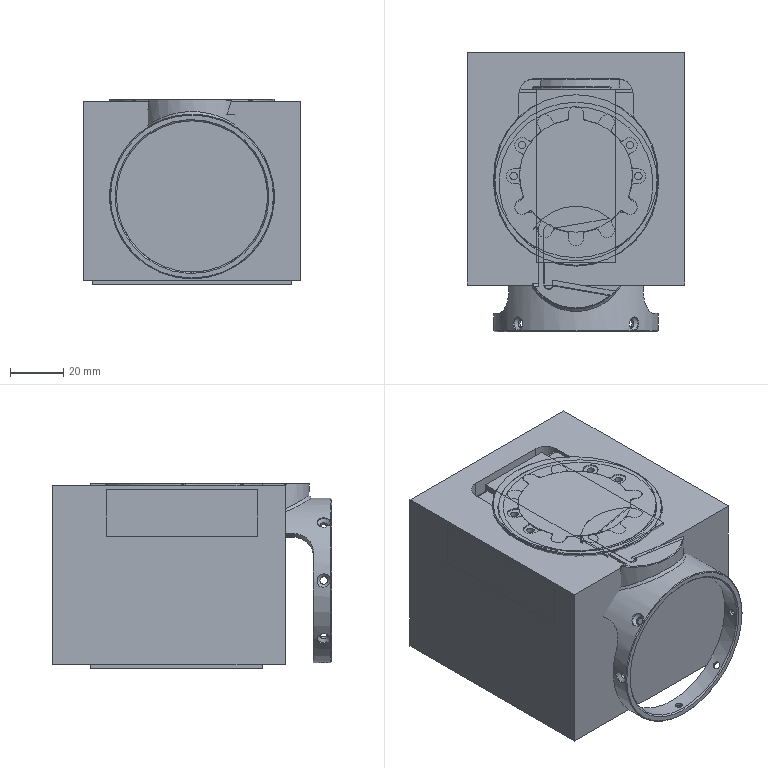NC program | NX | posted with a generic post | part box 82 x 105.2 x 70 mm
Lines 901 to 1807 of 123648:
(外形动态铣_COPY , TOOL : 粗刀D10)
N1782 T15 M6
N1784 G53
N1786 G18 G0 G90 X2.248 Z-25.338 S8500 M3
N1788 G43 Y78.5 H15
N1790 G94 G1 Y34.864 F3500.
N1792 X2.295 Y34.857 Z-25.155
N1794 X2.305 Y34.856 Z-25.13
N1796 X2.322 Y34.855 Z-25.11
N1798 X2.344 Y34.854 Z-25.095
N1800 X2.369 Y34.853 Z-25.088
N1802 X2.396 Y34.852
N1804 X2.421 Y34.851 Z-25.095
N1806 X2.443 Z-25.11
N1808 G3 X2.443 Y34.033 Z-25.11 I-2.424 K-2.83
N1810 X2.443 Y33.215 Z-25.11 I-2.424 K-2.83
N1812 X2.443 Y32.398 Z-25.11 I-2.424 K-2.83
N1814 X2.443 Y31.58 Z-25.11 I-2.424 K-2.83
N1816 X2.443 Y30.762 Z-25.11 I-2.424 K-2.83
N1818 X2.443 Y29.945 Z-25.11 I-2.424 K-2.83
N1820 X2.443 Y29.127 Z-25.11 I-2.424 K-2.83
N1822 X2.443 Y28.309 Z-25.11 I-2.424 K-2.83
N1824 X2.443 Y27.492 Z-25.11 I-2.424 K-2.83
N1826 X2.443 Y26.674 Z-25.11 I-2.424 K-2.83
N1828 X2.443 Y25.856 Z-25.11 I-2.424 K-2.83
N1830 X2.443 Y25.039 Z-25.11 I-2.424 K-2.83
N1832 X2.443 Y24.221 Z-25.11 I-2.424 K-2.83
N1834 X2.443 Y23.403 Z-25.11 I-2.424 K-2.83
N1836 X2.443 Y22.586 Z-25.11 I-2.424 K-2.83
N1838 X2.443 Y21.768 Z-25.11 I-2.424 K-2.83
N1840 X2.443 Y20.95 Z-25.11 I-2.424 K-2.83
N1842 X2.443 Y20.133 Z-25.11 I-2.424 K-2.83
N1844 X2.443 Y19.315 Z-25.11 I-2.424 K-2.83
N1846 X2.443 Y18.497 Z-25.11 I-2.424 K-2.83
N1848 X2.443 Y17.68 Z-25.11 I-2.424 K-2.83
N1850 X2.443 Y16.862 Z-25.11 I-2.424 K-2.83
N1852 X2.443 Y16.044 Z-25.11 I-2.424 K-2.83
N1854 X3.745 Y15.93 Z-28.001 R3.727
N1856 X3.745 Z-27.96 R-3.748
N1858 G1 X3.778 Z-28.081
N1860 X3.79 Z-28.205
N1862 X3.795 Z-28.231
N1864 G3 X1.945 Z-31.269 R3.792
N1866 X-2.771 Z-30.609 R3.819
N1868 X-3.768 Z-28.538 R3.906
N1870 X-0.169 Z-24.196 R3.816
N1872 X2.469 Z-25.105 R3.845
N1874 X3.293 Z-26.089 R4.24
N1876 X3.793 Z-28.262 R3.828
N1878 X3.166 Z-28.712 R0.505
N1880 G1 X1.594 Z-28.316
N1882 Y16.93
N1884 G0 Y78.5
N1886 X29.527 Z-4.88
N1888 G1 Y19.899
N1890 Y18.899
N1892 G3 X29.287 Z-5.852 R-0.505
N1894 G1 X27.657 Z-5.215
N1896 G3 X27.345 Z-4.842 R0.505
N1898 X27.07 Z-3.887 R14.618
N1900 G1 X27.042 Z-3.804
N1902 G3 X26.84 Z-3.011 R8.746
N1904 X26.876 Z-2.627 R0.799
N1906 G2 X27.225 Z-1.531 R5.794
N1908 G1 X27.344 Z-1.173
N1910 X27.352 Z-1.115
N1912 X27.344 Z-1.173
N1914 G2 X27.175 Z-1.747 R3.561
N1916 G3 X26.876 Z-2.627 R5.632
N1918 G2 X26.768 Z-3.082 R0.871
N1920 X26.918 Z-3.475 R1.353
N1922 G1 X27.042 Z-3.804
N1924 G2 X27.892 Z-3.962 R0.505
N1926 G1 X28.397 Z-3.393
N1928 G3 X29.279 Z-3.726 R0.505
N1930 G1 Y19.899
N1932 G0 Y78.5
N1934 X29.067 Z-5.02
N1936 G1 Y20.394
N1938 Y19.394
N1940 G3 X28.826 Z-5.992 R-0.505
N1942 G1 X27.198 Z-5.358
N1944 G3 X26.886 Z-4.985 R0.505
N1946 X26.719 Z-4.45 R15.136
N1948 G2 X26.532 Z-3.77 R4.464
N1950 G3 X26.34 Z-2.921 R8.059
N1952 X26.373 Z-2.645 R0.907
N1954 G2 X26.736 Z-1.479 R5.658
N1956 G1 X26.885 Z-1.03
N1958 X26.892 Z-0.971
N1960 X26.885 Z-1.03
N1962 G2 X26.68 Z-1.745 R4.244
N1964 G3 X26.373 Z-2.645 R5.523
N1966 G2 X26.275 Z-3.083 R0.804
N1968 X26.423 Z-3.475 R1.395
N1970 G1 X26.554 Z-3.827
N1972 G2 X27.379 Z-4.013 R0.505
N1974 G1 X27.953 Z-3.456
N1976 G3 X28.81 Z-3.815 R0.505
N1978 G1 Y20.394
N1980 G0 Y78.5
N1982 X28.656 Z-5.851
N1984 G1 Y20.888
N1986 Y19.888
N1988 G2 X28.744 Z-4.797 R-0.529
N1990 G1 X26.939 Z-4.685
N1992 G3 X26.48 Z-4.351 R0.529
N1994 G1 X26.468 Z-4.321
N1996 X26.167 Z-3.774
N1998 G3 X25.939 Z-2.813 R3.831
N2000 X26.012 Z-2.509 R0.818
N2002 G1 X26.47 Z-1.632
N2004 X26.48 Z-1.606
N2006 X26.47 Z-1.632
N2008 X26.012 Z-2.509
N2010 G2 X25.854 Z-3.04 R1.2
N2012 X25.983 Z-3.439 R0.961
N2014 G1 X26.224 Z-3.877
N2016 G2 X27.094 Z-3.904 R0.505
N2018 G1 X27.533 Z-3.208
N2020 G3 X28.465 Z-3.475 R0.505
N2022 G1 Y20.888
N2024 G0 Y78.5
N2026 X28.308 Z-4.565
N2028 G1 Y21.383
N2030 Y20.383
N2032 G2 X27.409 Z-4.22 R0.505
N2034 G1 X27.001 Z-4.732
N2036 G3 X26.132 Z-4.59 R0.505
N2038 X25.662 Z-3.658 R36.06
N2040 G1 X25.607 Z-3.452
N2042 G3 X25.532 Z-2.922 R2.623
N2044 G1 X25.548 Z-2.786
N2046 G2 X25.764 Z-1.296 R6.024
N2048 X25.744 Z0.158 R22.27
N2050 X23.618 Z3.888 R5.207
N2052 X22.281 Z4.703 R10.28
N2054 X21.487 Z4.989 R4.809
N2056 G3 X22.984 Z4.312 R5.372
N2058 X24.143 Z3.456 R8.234
N2060 X25.763 Z-0.441 R5.229
N2062 X25.742 Z-1.747 R17.885
N2064 X25.548 Z-2.786 R6.162
N2066 G2 X25.536 Z-3.207 R0.736
N2068 G1 X25.607 Z-3.452
N2070 G2 X26.03 Z-3.813 R0.505
N2072 G1 X27.616 Z-4.01
N2074 G2 X27.767 Z-3.012 R0.505
N2076 G1 Y21.383
N2078 G0 Y78.5
N2080 X30.042 Z-58.825
N2082 G1 Y19.404
N2084 Y18.404
N2086 G3 X30.341 Z-59.935 R0.586
N2088 G1 X28.506 Z-60.856
N2090 G3 X27.814 Z-60.731 R0.586
N2092 X27.604 Z-60.279 R2.401
N2094 X27.657 Z-59.848 R0.81
N2096 G1 X27.8 Z-59.618
N2098 X27.81 Z-59.595
N2100 X27.8 Z-59.618
N2102 X27.591 Z-59.954
N2104 G2 X27.48 Z-60.428 R1.361
N2106 X27.604 Z-60.774 R0.524
N2108 X27.868 Z-60.989 R0.65
N2110 G1 X27.849 Z-60.986
N2112 X27.835 Z-60.983
N2114 X27.814 Z-60.976
N2116 G3 X27.494 Z-60.109 R0.566
N2118 G1 X27.626 Z-59.897
N2120 G3 X27.85 Z-59.699 R0.529
N2122 G1 X29.985 Z-58.695
N2124 Y19.404
N2126 G0 Y78.5
N2128 X29.567 Z-58.825
N2130 G1 Y19.899
N2132 Y18.899
N2134 G3 X29.437 Z-59.234 R0.586
N2136 G1 X28.234 Z-60.714
N2138 G3 X27.349 Z-60.742 R0.586
N2140 X27.146 Z-60.32 R2.797
N2142 X27.174 Z-59.848 R0.752
N2144 G1 X27.335 Z-59.584
N2146 X27.345 Z-59.558
N2148 X27.335 Z-59.584
N2150 X27.11 Z-59.955
N2152 G2 X27.017 Z-60.539 R1.208
N2154 X27.457 Z-60.998 R0.662
N2156 G1 X27.349 Z-60.98
N2158 G3 X27.013 Z-60.116 R0.567
N2160 G1 X27.142 Z-59.902
N2162 G3 X27.663 Z-59.65 R0.531
N2164 G1 X29.497 Z-59.882
N2166 G2 X29.567 Z-58.825 R-0.531
N2168 G1 Y19.899
N2170 G0 Y78.5
N2172 X29.202 Z-58.823
N2174 G1 Y20.394
N2176 Y19.394
N2178 G3 X29.058 Z-59.256 R0.605
N2180 G1 X27.786 Z-60.746
N2182 G3 X26.892 Z-60.774 R0.605
N2184 X26.577 Z-60.022 R2.95
N2186 X26.584 Z-59.73 R1.193
N2188 G2 X26.73 Z-59.172 R8.097
N2190 G1 X26.884 Z-58.682
N2192 X26.892 Z-58.621
N2194 X26.884 Z-58.682
N2196 G2 X26.613 Z-59.643 R8.144
N2198 G1 X26.543 Z-59.848
N2200 G2 X26.495 Z-60.558 R1.711
N2202 X26.945 Z-61. R0.664
N2204 G1 X26.892 Z-60.997
N2206 X26.744 Z-60.967
N2208 G3 X26.391 Z-60.481 R0.64
N2210 G1 X26.383 Z-60.293
N2212 X26.555 Z-59.815
N2214 X26.383 Z-60.293
N2216 G2 X26.744 Z-60.967 R0.561
N2218 X27.157 Z-60.941 R0.636
N2220 G1 X29.309 Z-60.045
N2222 G2 X29.092 Z-58.823 R0.636
N2224 G1 Y20.394
N2226 G0 Y78.5
N2228 X28.792
N2230 G1 Y20.888
N2232 Y19.888
N2234 G3 X28.627 Z-59.287 R0.623
N2236 G1 X27.243 Z-60.783
N2238 G3 X26.462 Z-60.893 R0.623
N2240 X26.314 Z-60.693 R0.578
N2242 X26.072 Z-59.911 R4.395
N2244 X26.093 Z-59.648 R0.932
N2246 G2 X26.277 Z-58.716 R5.664
N2248 G3 X26.478 Z-58.083 R7.143
N2250 G1 X26.485 Z-58.025
N2252 X26.478 Z-58.083
N2254 G2 X26.277 Z-58.716 R7.143
N2256 G3 X26.093 Z-59.648 R5.664
N2258 G1 X26.013 Z-59.885
N2260 G2 X26.012 Z-60.517 R1.917
N2262 X26.295 Z-60.91 R0.55
N2264 G1 X26.503 Z-61.
N2266 X26.431
N2268 X26.374 Z-60.997
N2270 X26.352 Z-60.995
N2272 X26.235 Z-60.953
N2274 G3 X25.972 Z-60.681 R1.494
N2276 X25.889 Z-60.321 R0.58
N2278 G1 X25.911 Z-60.157
N2280 X25.947 Z-60.075
N2282 X25.957 Z-60.051
N2284 X26.037 Z-59.814
N2286 X25.957 Z-60.051
N2288 X25.947 Z-60.075
N2290 X25.911 Z-60.157
N2292 G2 X26.352 Z-60.995 R0.573
N2294 X26.641 Z-60.949 R0.631
N2296 G1 X28.846 Z-60.036
N2298 G2 X28.64 Z-58.823 R0.631
N2300 G1 Y20.888
N2302 G0 Y78.5
N2304 X28.363 Z-58.825
N2306 G1 Y21.383
N2308 Y20.383
N2310 G3 X28.632 Z-60.019 R0.622
N2312 G1 X26.416 Z-60.955
N2314 G3 X26.004 Z-60.917 R0.46
N2316 G1 X25.908 Z-60.836
N2318 G3 X25.742 Z-60.423 R1.485
N2320 X25.584 Z-59.686 R7.721
N2322 G1 X25.585 Z-59.522
N2324 G2 X25.763 Z-58.404 R5.443
N2326 G1 X25.795 Z-58.269
N2328 X26.13 Z-57.261
N2330 X26.138 Z-57.203
N2332 X26.13 Z-57.261
N2334 X25.776 Z-58.338
N2336 G2 X25.731 Z-58.775 R4.176
N2338 G3 X25.585 Z-59.522 R5.461
N2340 G1 X25.563 Z-59.618
N2342 X25.555 Z-59.644
N2344 X25.514 Z-59.763
N2346 G2 X25.568 Z-60.625 R1.514
N2348 X25.923 Z-60.955 R0.574
N2350 G1 X26.074 Z-61.
N2352 X26.199
N2354 X25.949
N2356 X25.826 Z-60.977
N2358 X25.627 Z-60.839
N2360 G3 X25.417 Z-60.541 R1.294
N2362 X25.384 Z-60.129 R0.836
N2364 G1 X25.408 Z-60.07
N2366 X25.413 Z-60.057
N2368 X25.535 Z-59.702
N2370 X25.413 Z-60.057
N2372 X25.408 Z-60.07
N2374 X25.384 Z-60.129
N2376 G2 X25.478 Z-60.836 R0.609
N2378 X25.891 Z-61. R0.589
N2380 G1 X26.016
N2382 G2 X26.459 Z-60.795 R0.582
N2384 G1 X27.812 Z-59.201
N2386 G2 X27.951 Z-58.825 R0.582
N2388 G1 Y21.383
N2390 G0 Y78.5
N2392 X28.115 Z-58.823
N2394 G1 Y21.878
N2396 Y20.878
N2398 G3 X28.369 Z-60.051 R0.636
N2400 G1 X26.012 Z-60.958
N2402 G3 X25.446 Z-60.892 R0.605
N2404 G1 X25.294 Z-60.683
N2406 G3 X25.087 Z-59.212 R7.832
N2408 G2 X25.187 Z-57.904 R5.906
N2410 G1 X25.193 Z-3.464
N2412 G2 X25.178 Z0.004 R213.685
N2414 X23.973 Z3.026 R5.21
N2416 X22.723 Z4.106 R5.746
N2418 X21.598 Z4.749 R7.672
N2420 X20.859 Z5.003 R5.58
N2422 G3 X20.981 Z5.987 R0.5
N2424 G1 X21.893
N2426 X23.493 Y21.378
N2428 X24.17 Z5.984 F15000.
N2430 X24.336 Z5.934
N2432 X24.907 Z5.653
N2434 X25.469 Z5.353
N2436 G3 X26.515 Z4.119 R2.718
N2438 G1 X27.493 Z1.804
N2440 G3 X28.263 Z-2.383 R11.082
N2442 G1 X27.628 Z-56.727
N2444 G3 X27.46 Z-57.039 R0.511
N2446 G1 X27.191 Z-57.271
N2448 X25.98 Y20.878 Z-58.317 F3500.
N2450 X25.246 Z-58.952
N2452 G2 X25.087 Z-59.212 R0.5
N2454 G1 X24.988 Z-59.621
N2456 X24.982 Z-59.642
N2458 G2 X24.96 Z-60.397 R1.665
N2460 X25.098 Z-60.736 R1.339
N2462 X25.516 Z-60.986 R0.616
N2464 G1 X25.566 Z-61.
N2466 X25.816
N2468 X25.441
N2470 X25.318 Z-60.981
N2472 X25.108 Z-60.847
N2474 G3 X24.878 Z-60.548 R1.841
N2476 X24.858 Z-60.015 R0.726
N2478 G1 X24.878 Z-59.958
N2480 X24.882 Z-59.948
N2482 X24.982 Z-59.642
N2484 X24.882 Z-59.948
N2486 X24.878 Z-59.958
N2488 X24.842 Z-60.055
N2490 X24.836 Z-60.071
N2492 X24.789 Z-60.178
N2494 X24.76 Z-60.299
N2496 G2 X24.832 Z-60.659 R1.287
N2498 X25.092 Z-60.921 R0.564
N2500 G1 X25.279 Z-60.998
N2502 X25.318 Z-61.
N2504 X25.443
N2506 X25.318
N2508 X25.279 Z-60.998
N2510 G3 X24.789 Z-60.178 R0.569
N2512 X25.048 Z-59.908 R0.588
N2514 G1 X27.339 Z-58.714
N2516 Y21.878
N2518 G0 Y78.5
N2520 X27.499 Z-58.823
N2522 G1 Y22.373
N2524 Y21.373
N2526 G3 X27.756 Z-60.034 R0.628
N2528 G1 X25.451 Z-60.955
N2530 G3 X24.878 Z-60.902 R0.633
N2532 G1 X24.724 Z-60.702
N2534 G3 X24.526 Z-59.641 R7.264
N2536 X24.494 Z-59.174 R1.883
N2538 G2 X24.588 Z-57.904 R5.87
N2540 G1 X24.595 Z-32.861
N2542 G3 X24.66 Z-31.981 R7.101
N2544 G2 X24.679 Z-24.203 R39.152
N2546 G1 X24.595 Z-23.298
N2548 X24.588 Z-0.441
N2550 G2 X22.29 Z3.991 R5.19
N2552 X21.413 Z4.536 R17.777
N2554 X20.188 Z5.015 R5.079
N2556 G3 X20.153 Z5.965 R0.5
N2558 G1 X20.294 Z6.017
N2560 X21.796 Y21.873 Z6.569
N2562 X22.84 Z6.948 F15000.
N2564 G3 X23.306 Z6.815 R0.503
N2566 G1 X26.557 Z3.557
N2568 G3 X27.306 Z1.608 R2.915
N2570 G1 X27.303 Z-14.519
N2572 X27.28 Z-23.185
N2574 X27.234 Z-31.852
N2576 X27.035 Z-56.69
N2578 G3 X26.863 Z-57.006 R0.51
N2580 G1 X26.592 Z-57.236
N2582 X25.371 Y21.373 Z-58.27 F3500.
N2584 X24.665 Z-58.87
N2586 G2 X24.494 Z-59.174 R0.5
N2588 G3 X24.382 Z-59.641 R4.804
N2590 G2 X24.48 Z-60.692 R1.54
N2592 X24.875 Z-60.976 R0.596
N2594 G1 X24.964 Z-61.
N2596 X25.339
N2598 X24.839
N2600 X24.716 Z-60.979
N2602 X24.503 Z-60.832
N2604 G3 X24.285 Z-60.553 R1.705
N2606 X24.252 Z-60.025 R0.725
N2608 G1 X24.382 Z-59.641
N2610 X24.244 Z-60.051
N2612 X24.234 Z-60.075
N2614 X24.189 Z-60.177
N2616 X24.16 Z-60.299
N2618 G2 X24.231 Z-60.653 R1.378
N2620 X24.487 Z-60.918 R0.562
N2622 G1 X24.677 Z-60.998
N2624 X24.718 Z-61.
N2626 X24.843
N2628 X24.718
N2630 X24.677 Z-60.998
N2632 G3 X24.189 Z-60.177 R0.569
N2634 X24.447 Z-59.909 R0.589
N2636 G1 X26.741 Z-58.703
N2638 Y22.373
N2640 G0 Y78.5
N2642 X26.889 Z-58.823
N2644 G1 Y22.868
N2646 Y21.868
N2648 G3 X27.147 Z-60.031 R0.627
N2650 G1 X24.852 Z-60.955
N2652 G3 X24.278 Z-60.902 R0.633
N2654 G1 X24.124 Z-60.702
N2656 G3 X23.926 Z-59.641 R7.224
N2658 G1 X23.871 Z-59.137
N2660 G2 X23.962 Z-57.903 R5.538
N2662 G1 X23.964 Z-35.457
N2664 G3 X24.063 Z-34.573 R3.822
N2666 G2 X24.466 Z-31.548 R39.464
N2668 X24.675 Z-28.95 R47.216
N2670 X24.603 Z-25.933 R25.491
N2672 X24.23 Z-22.475 R64.034
N2674 G1 X24.014 Z-21.141
N2676 X23.965 Z-20.693
N2678 X23.962 Z-0.441
N2680 G2 X22.283 Z3.506 R5.217
N2682 X21.418 Z4.149 R6.
N2684 X20.327 Z4.749 R9.712
N2686 X19.594 Z5.001 R6.662
N2688 G3 X19.543 Z5.957 R0.5
N2690 G1 X19.681 Z6.007
N2692 X21.185 Y22.368 Z6.553
N2694 X22.248 Z6.935 F15000.
N2696 G3 X22.712 Z6.801 R0.503
N2698 G1 X25.946 Z3.562
N2700 G3 X26.726 Z1.576 R3.01
N2702 G1 X26.951 Z-17.779
N2704 G3 X26.753 Z-42.894 R755.168
N2706 G1 X26.411 Z-56.651
N2708 G3 X26.241 Z-56.96 R0.511
N2710 G1 X25.965 Z-57.195
N2712 X24.748 Y21.868 Z-58.233 F3500.
N2714 X24.04 Z-58.836
N2716 G2 X23.871 Z-59.137 R0.5
N2718 G1 X23.754 Z-59.643
N2720 G2 X23.856 Z-60.675 R1.627
N2722 X24.365 Z-60.993 R0.62
N2724 G1 X24.39 Z-61.
N2726 X24.64
N2728 X24.265
N2730 X24.14 Z-60.988
N2732 X23.93 Z-60.87
N2734 G3 X23.634 Z-60.484 R1.37
N2736 X23.61 Z-60.07 R0.817
N2738 G1 X23.615 Z-60.056
N2740 X23.754 Z-59.643
N2742 X23.615 Z-60.056
N2744 X23.61 Z-60.07
N2746 X23.587 Z-60.129
N2748 X23.581 Z-60.142
N2750 X23.568 Z-60.17
N2752 X23.539 Z-60.292
N2754 G2 X23.607 Z-60.642 R1.435
N2756 X23.858 Z-60.913 R0.56
N2758 G1 X24.053 Z-60.998
N2760 X24.095 Z-61.
N2762 X24.345
N2764 X24.095
N2766 X24.053 Z-60.998
N2768 G3 X23.568 Z-60.17 R0.569
N2770 X23.823 Z-59.91 R0.587
N2772 G1 X26.114 Z-58.714
N2774 Y22.868
N2776 G0 Y78.5
N2778 X26.247 Z-58.823
N2780 G1 Y23.362
N2782 Y22.362
N2784 G3 X26.215 Z-59.911 R0.625
N2786 G1 X24.281 Z-60.928
N2788 G3 X23.651 Z-60.895 R0.615
N2790 G1 X23.499 Z-60.698
N2792 G3 X23.302 Z-59.639 R7.309
N2794 G1 X23.226 Z-59.004
N2796 G2 X23.294 Z-57.904 R5.912
N2798 G1 X23.297 Z-37.231
N2800 G3 X23.467 Z-36.302 R5.471
N2802 G2 X23.821 Z-34.551 R40.838
N2804 X24.448 Z-31.444 R31.314
N2806 X23.843 Z-21.579 R24.764
N2808 X23.425 Z-19.517 R37.831
N2810 G3 X23.3 Z-18.726 R13.405
N2812 G1 X23.294 Z-0.441
N2814 G2 X20.985 Z3.999 R5.193
N2816 X19.641 Z4.749 R11.461
N2818 X18.959 Z4.994 R6.353
N2820 G3 X19.056 Z5.985 R0.5
N2822 G1 X19.976 Z5.983
N2824 X21.576 Y22.862 Z5.98
N2826 X22.271 Z5.975 F15000.
N2828 X22.436 Z5.926
N2830 X23.007 Z5.645
N2832 X23.568 Z5.344
N2834 G3 X24.605 Z4.107 R2.669
N2836 G1 X25.555 Z1.78
N2838 G3 X26.252 Z-2.356 R10.761
N2840 G1 X25.84 Z-16.242
N2842 G3 X25.662 Z-16.554 R0.51
N2844 G1 X25.302 Z-16.846
N2846 X24.061 Y22.362 Z-17.855 F3500.
N2848 X23.485 Z-18.324
N2850 G2 X23.3 Z-18.726 R0.5
N2852 X23.328 Z-19.099 R1.646
N2854 G1 X23.437 Z-19.572
N2856 G2 X23.735 Z-19.924 R0.5
N2858 G1 X24.238 Z-20.131
N2860 X25.718 Y22.862 Z-20.739
N2862 X26.302 Z-20.982 F15000.
N2864 G3 X26.555 Z-21.372 R0.503
N2866 G1 X26.748 Z-23.407
N2868 X26.919 Z-25.443
N2870 G3 X26.971 Z-30.339 R43.519
N2872 G1 X25.765 Z-56.517
N2874 G3 X25.597 Z-56.816 R0.513
N2876 G1 X25.295 Z-57.074
N2878 X24.08 Y22.362 Z-58.115 F3500.
N2880 X23.395 Z-58.701
N2882 G2 X23.226 Z-59.004 R0.5
N2884 G3 X23.094 Z-59.621 R3.815
N2886 G2 X23.212 Z-60.657 R1.674
N2888 X23.71 Z-60.991 R0.611
N2890 G1 X23.743 Z-61.
N2892 X24.118
N2894 X23.618
N2896 X23.494 Z-60.986
N2898 X23.279 Z-60.856
N2900 G3 X22.975 Z-60.452 R1.582
N2902 X22.95 Z-60.04 R0.832
N2904 G1 X23.087 Z-59.641
N2906 X23.094 Z-59.621
N2908 X22.893 Z-60.19
N2910 G2 X22.968 Z-60.671 R1.175
N2912 X23.234 Z-60.927 R0.565
N2914 G1 X23.423 Z-61.
N2916 X23.673
N2918 X23.423
N2920 G3 X22.891 Z-60.18 R0.572
N2922 G1 X22.938 Z-60.073
N2924 G3 X23.21 Z-59.788 R0.574
N2926 G1 X25.448 Z-58.686
N2928 Y23.362
N2930 G0 Y78.5
N2932 X25.562 Z-58.823
N2934 G1 Y23.857
N2936 Y22.857
N2938 G3 X25.538 Z-59.911 R0.623
N2940 G1 X23.611 Z-60.928
N2942 G3 X22.981 Z-60.896 R0.616
N2944 G1 X22.827 Z-60.697
N2946 G3 X22.631 Z-59.642 R7.117
N2948 X22.543 Z-58.831 R14.807
N2950 G2 X22.585 Z-57.903 R6.27
N2952 G1 X22.592 Z-38.939
N2954 G3 X22.764 Z-38.03 R3.172
N2956 G1 X23.117 Z-36.699
N2958 G2 X24.118 Z-33.278 R28.314
N2960 X23.143 Z-19.387 R24.753
N2962 G1 X22.835 Z-18.224
N2964 G3 X22.592 Z-16.75 R13.55
N2966 G1 X22.585 Z-0.441
N2968 G2 X21.367 Z3.025 R5.21
N2970 X19.751 Z4.313 R5.59
N2972 X18.826 Z4.786 R7.766
N2974 X18.197 Z4.998 R5.071
N2976 G3 X18.137 Z5.956 R0.5
N2978 G1 X18.27 Z6.004
N2980 X19.775 Y23.357 Z6.548
N2982 X20.852 Z6.933 F15000.
N2984 G3 X21.315 Z6.798 R0.503
N2986 G1 X24.577 Z3.531
N2988 G3 X25.303 Z1.608 R2.833
N2990 G1 X25.133 Z-14.266
N2992 G3 X24.953 Z-14.586 R0.509
N2994 G1 X24.6 Z-14.874
N2996 X23.36 Y22.857 Z-15.886 F3500.
N2998 X22.776 Z-16.362
N3000 G2 X22.592 Z-16.75 R0.5
N3002 X22.614 Z-17.383 R3.663
N3004 X22.848 Z-18.276 R10.518
N3006 X23.763 Z-18.413 R0.505
N3008 G1 X24.123 Z-17.842
N3010 G3 X25.055 Z-18.106 R0.505
N3012 G1 Y23.857
N3014 G0 Y78.5
N3016 X24.831 Z-58.823
N3018 G1 Y23.857
N3020 Y22.857
N3022 G3 X24.757 Z-59.133 R0.528
N3024 G1 X23.789 Z-60.744
N3026 G3 X23.336 Z-61. R0.528
N3028 G1 X23.211
N3030 G3 X22.972 Z-60.935 R0.541
N3032 X22.545 Z-60.39 R1.862
N3034 G1 X22.435 Z-60.175
N3036 G3 X22.369 Z-59.669 R0.744
N3038 G2 X22.546 Z-58.817 R4.874
N3040 G3 X22.369 Z-59.669 R4.874
N3042 G1 X22.331 Z-59.788
N3044 X22.303 Z-59.91
N3046 G2 X22.494 Z-60.708 R1.586
N3048 X22.898 Z-60.98 R0.603
N3050 G1 X22.97 Z-61.
N3052 X23.22
N3054 X22.845
N3056 X22.722 Z-60.979
N3058 X22.519 Z-60.848
N3060 G3 X22.278 Z-60.555 R1.908
N3062 X22.232 Z-60.07 R0.723
N3064 G1 X22.366 Z-59.678
N3066 X22.232 Z-60.07
N3068 X22.185 Z-60.178
N3070 X22.156 Z-60.299
N3072 G2 X22.225 Z-60.648 R1.268
N3074 X22.479 Z-60.916 R0.561
N3076 G1 X22.671 Z-60.998
N3078 X22.714 Z-61.
N3080 X22.964
N3082 X22.714
N3084 X22.671 Z-60.998
N3086 G3 X22.185 Z-60.178 R0.569
N3088 X22.451 Z-59.906 R0.583
N3090 G1 X24.733 Z-58.765
N3092 Y23.857
N3094 G0 Y78.5
N3096 X24.836 Z-58.823
N3098 G1 Y24.352
N3100 Y23.352
N3102 G3 X24.82 Z-59.909 R0.62
N3104 G1 X22.905 Z-60.928
N3106 G3 X22.274 Z-60.902 R0.628
N3108 G1 X22.119 Z-60.702
N3110 G3 X21.922 Z-59.642 R7.204
N3112 X21.813 Z-58.624 R21.224
N3114 G2 X21.834 Z-57.903 R5.787
N3116 G1 X21.843 Z-40.22
N3118 G3 X21.944 Z-39.757 R1.197
N3120 G1 X22.373 Z-38.445
N3122 G3 X22.655 Z-37.844 R6.373
N3124 G1 X22.913 Z-37.458
N3126 G2 X23.117 Z-36.699 R10.669
N3128 X24.118 Z-33.278 R28.314
N3130 X23.143 Z-19.387 R24.753
N3132 G1 X22.919 Z-18.538
N3134 G2 X22.598 Z-18.041 R7.171
N3136 G3 X22.211 Z-17.048 R6.241
N3138 X21.842 Z-14.831 R13.553
N3140 G1 X21.834 Z-0.441
N3142 G2 X19.256 Z4.162 R5.189
N3144 X17.958 Z4.822 R11.328
N3146 G1 X17.433 Z4.996
N3148 G3 X17.37 Z5.955 R0.5
N3150 G1 X17.499 Z6.001
N3152 X19.004 Y23.852 Z6.544
N3154 X20.088 Z6.93 F15000.
N3156 G3 X20.55 Z6.796 R0.503
N3158 G1 X23.813 Z3.528
N3160 G3 X24.538 Z1.606 R2.831
N3162 G1 X24.383 Z-12.348
N3164 G3 X24.204 Z-12.667 R0.509
N3166 G1 X23.847 Z-12.958
N3168 X22.607 Y23.352 Z-13.969 F3500.
N3170 X22.026 Z-14.443
N3172 G2 X21.842 Z-14.831 R0.5
N3174 X21.859 Z-15.937 R16.442
N3176 X22.007 Z-16.426 R3.027
N3178 G1 X22.227 Z-17.096
N3180 G2 X23.148 Z-17.19 R0.505
N3182 G1 X23.492 Z-16.58
N3184 G3 X24.436 Z-16.823 R0.505
N3186 G1 Y24.352
N3188 G0 Y78.5
N3190 X24.098 Z-58.823
N3192 G1 Y24.352
N3194 Y23.352
N3196 G3 X24.027 Z-59.126 R0.525
N3198 G1 X23.083 Z-60.74
N3200 G3 X22.629 Z-61. R0.525
N3202 G1 X22.504
N3204 G3 X22.264 Z-60.936 R0.539
N3206 X21.836 Z-60.389 R1.865
N3208 X21.63 Z-59.94 R2.331
N3210 X21.626 Z-59.645 R0.871
N3212 G2 X21.821 Z-58.506 R4.888
N3214 G3 X21.626 Z-59.645 R4.888
N3216 G1 X21.586 Z-59.764
N3218 G2 X21.577 Z-60.136 R1.075
N3220 X21.784 Z-60.723 R1.711
N3222 X22.196 Z-60.983 R0.609
N3224 G1 X22.255 Z-61.
N3226 X22.505
N3228 X22.13
N3230 X22.007 Z-60.98
N3232 G3 X21.557 Z-60.573 R1.257
N3234 X21.48 Z-60.076 R0.732
N3236 G1 X21.482 Z-60.071
N3238 X21.488 Z-60.055
N3240 X21.608 Z-59.7
N3242 X21.488 Z-60.055
N3244 X21.482 Z-60.071
N3246 X21.434 Z-60.188
N3248 X21.41 Z-60.31
N3250 G2 X21.496 Z-60.659 R1.269
N3252 X21.755 Z-60.921 R0.562
N3254 G1 X21.946 Z-60.999
N3256 X21.968 Z-61.
N3258 X22.218
N3260 X21.968
N3262 X21.946 Z-60.999
N3264 G3 X21.434 Z-60.188 R0.57
N3266 X21.711 Z-59.9 R0.581
N3268 G1 X23.981 Z-58.793
N3270 Y24.352
N3272 G0 Y78.5
N3274 X24.065 Z-58.823
N3276 G1 Y24.847
N3278 Y23.847
N3280 G3 X23.877 Z-59.308 R0.616
N3282 G1 X22.295 Z-60.828
N3284 G3 X21.528 Z-60.896 R0.613
N3286 G1 X21.374 Z-60.697
N3288 G3 X21.176 Z-59.637 R7.319
N3290 X21.034 Z-58.254 R24.101
N3292 G1 X21.047 Z-41.434
N3294 X21.094 Z-41.246
N3296 X21.484 Z-40.232
N3298 G3 X21.92 Z-39.387 R8.71
N3300 G1 X22.172 Z-39.047
N3302 X22.197 Z-38.995
N3304 G3 X23.131 Z-39.075 R0.5
N3306 G1 X23.519 Y24.347 Z-40.627
N3308 X23.767 Z-41.63 F15000.
N3310 X23.772 Z-41.723
N3312 X23.256 Z-56.089
N3314 G3 X23.039 Z-56.428 R0.518
N3316 G1 X21.784 Y23.847 Z-57.421 F3500.
N3318 X21.224 Z-57.865
N3320 G2 X21.034 Z-58.254 R0.5
N3322 G3 X20.905 Z-59.331 R4.75
N3324 G2 X20.897 Z-60.236 R2.225
N3326 X21.137 Z-60.778 R1.471
N3328 X21.576 Z-60.993 R0.643
N3330 G1 X21.601 Z-61.
N3332 X21.976
N3334 X21.476
N3336 X21.352 Z-60.988
N3338 X21.128 Z-60.863
N3340 G3 X20.758 Z-60.378 R1.549
N3342 X20.721 Z-59.957 R0.825
N3344 G1 X20.828 Z-59.643
N3346 X20.835 Z-59.619
N3348 X20.924 Z-59.254
N3350 X20.835 Z-59.619
N3352 X20.828 Z-59.643
N3354 X20.688 Z-60.054
N3356 X20.681 Z-60.072
N3358 X20.656 Z-60.195
N3360 G2 X20.84 Z-60.763 R1.094
N3362 X21.281 Z-61. R0.731
N3364 G1 X21.531
N3366 X21.164
N3368 X21.111 Z-60.998
N3370 X21.094 Z-60.996
N3372 G3 X20.609 Z-60.487 R0.609
N3374 G1 X20.599 Z-60.294
N3376 G3 X20.681 Z-60.072 R0.979
N3378 G2 X20.599 Z-60.294 R0.979
N3380 X21.094 Z-60.996 R0.563
N3382 X21.603 Z-60.775 R0.605
N3384 G1 X23.197 Z-58.823
N3386 Y24.847
N3388 G0 Y78.5
N3390 X23.246
N3392 G1 Y25.341
N3394 Y24.341
N3396 G3 X23.061 Z-59.303 R0.614
N3398 G1 X21.491 Z-60.827
N3400 G3 X20.724 Z-60.895 R0.61
N3402 G1 X20.572 Z-60.699
N3404 G3 X20.375 Z-59.64 R7.195
N3406 X20.18 Z-57.391 R28.814
N3408 G1 X20.184 Z-42.756
N3410 G3 X20.248 Z-42.469 R0.707
N3412 G1 X20.658 Z-41.544
N3414 G3 X21.148 Z-40.755 R11.257
N3416 G1 X21.39 Z-40.46
N3418 X21.417 Z-40.409
N3420 G3 X22.319 Z-40.446 R0.5
N3422 G1 X22.333 Y24.353 Z-40.482
N3424 X22.344 Y24.365 Z-40.519
N3426 X22.722 Y24.841 Z-41.995
N3428 X22.987 Z-43.038 F15000.
N3430 X22.992 Z-43.137
N3432 X22.4 Z-55.224
N3434 G3 X22.182 Z-55.56 R0.52
N3436 G1 X20.929 Y24.341 Z-56.554 F3500.
N3438 X20.369 Z-57.
N3440 G2 X20.18 Z-57.391 R0.5
N3442 G3 X20.148 Z-58.759 R14.059
N3444 G1 X20.079 Z-59.209
N3446 G2 X20.058 Z-60.163 R2.492
N3448 X20.281 Z-60.73 R1.763
N3450 X20.696 Z-60.985 R0.613
N3452 G1 X20.751 Z-61.
N3454 X21.126
N3456 X20.626
N3458 X20.502 Z-60.981
N3460 G3 X20.126 Z-60.686 R1.149
N3462 X19.925 Z-60.369 R2.712
N3464 X19.903 Z-59.844 R0.739
N3466 G1 X19.971 Z-59.643
N3468 X19.978 Z-59.62
N3470 X20.079 Z-59.209
N3472 X19.978 Z-59.62
N3474 X19.971 Z-59.643
N3476 X19.832 Z-60.053
N3478 X19.825 Z-60.073
N3480 X19.809 Z-60.197
N3482 G2 X20.026 Z-60.783 R1.147
N3484 X20.463 Z-61. R0.722
N3486 G1 X20.713
N3488 X20.308
N3490 X20.186 Z-60.973
N3492 G3 X19.897 Z-60.762 R1.184
N3494 X19.761 Z-60.419 R0.566
N3496 G1 X19.764 Z-60.223
N3498 X19.778 Z-60.184
N3500 X19.825 Z-60.073
N3502 X19.778 Z-60.184
N3504 X19.764 Z-60.223
N3506 G2 X20.308 Z-61. R0.568
N3508 X20.754 Z-60.781 R0.598
N3510 G1 X22.36 Z-58.823
N3512 Y25.341
N3514 G0 Y78.5
N3516 X22.364 Z-58.825
N3518 G1 Y25.836
N3520 Y24.836
N3522 G3 X22.367 Z-59.896 R0.61
N3524 G1 X20.503 Z-60.924
N3526 G3 X19.868 Z-60.896 R0.608
N3528 G1 X19.715 Z-60.698
N3530 G3 X19.518 Z-59.64 R7.199
N3532 X19.273 Z-56.226 R35.81
N3534 G1 X19.255 Z-55.651
N3536 X19.263 Z-43.943
N3538 G3 X19.344 Z-43.618 R0.738
N3540 X19.815 Z-42.728 R14.598
N3542 G1 X20.218 Z-42.183
N3544 X20.512 Z-41.862
N3546 X20.541 Z-41.813
N3548 G3 X21.413 Z-41.834 R0.5
N3550 G1 X21.436 Y24.854 Z-41.886
N3552 X21.454 Y24.872 Z-41.94
N3554 X21.835 Y25.336 Z-43.377
N3556 X22.112 Z-44.431 F15000.
N3558 X22.116 Z-44.541
N3560 X21.474 Z-53.482
N3562 G3 X21.258 Z-53.808 R0.523
N3564 G1 X20.009 Y24.836 Z-54.807 F3500.
N3566 X19.442 Z-55.261
N3568 G2 X19.255 Z-55.651 R0.5
N3570 G1 X19.253 Z-57.903
N3572 G3 X19.15 Z-59.21 R5.734
N3574 G2 X19.2 Z-60.299 R2.517
N3576 X19.499 Z-60.83 R1.393
N3578 X19.885 Z-61. R0.826
N3580 G1 X20.26
N3582 X19.76
N3584 X19.636 Z-60.984
N3586 G3 X19.254 Z-60.704 R1.129
N3588 X18.965 Z-60.176 R1.375